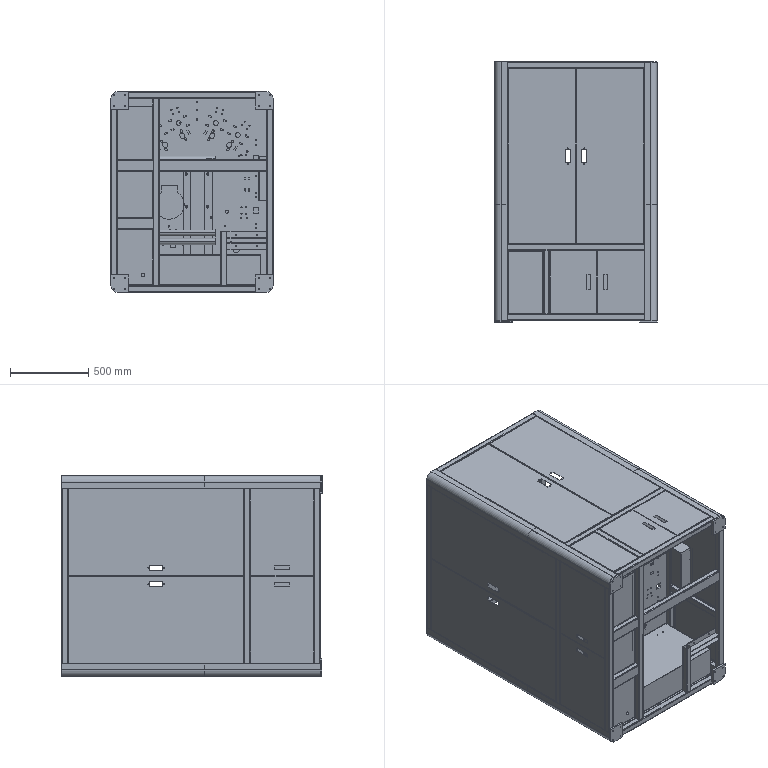Part | 78 solids | 2359 faces | box 1036 x 1664 x 1280 mm | volume 49269929 mm3 | plane 1352 | cylinder 888 | spline 119 | commonest cylinder face diameters 6.8 x138 8 x82 9 x69 10 x60 1.473 x57 3.3 x48